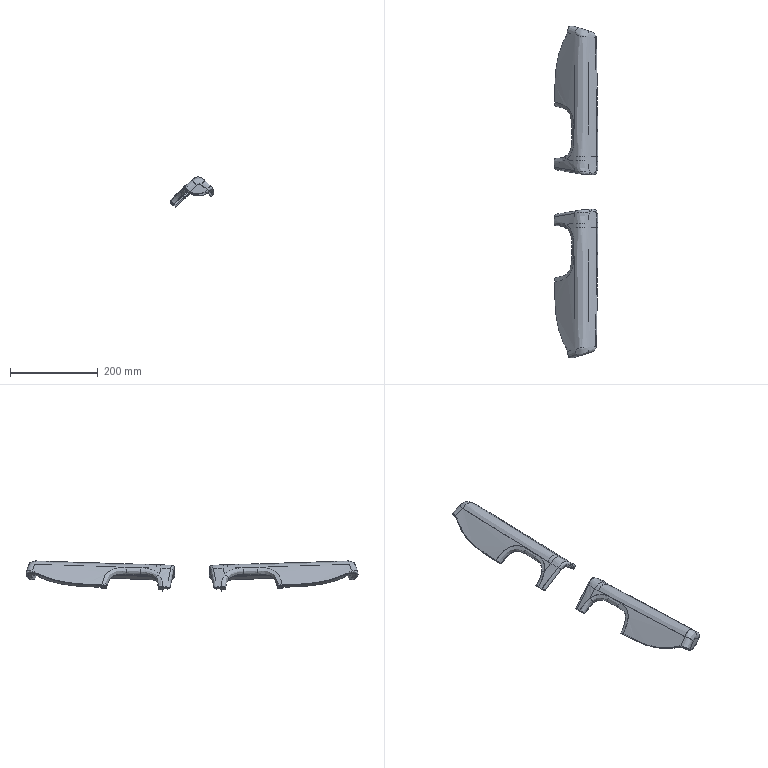Part | STEP file | L0193019AA ARMREST FRT DR MANUAL RH!SKIN VINYL ARMREST FRONT DOOR RH MANUAL | 2 solids | 636 faces | box 99.664 x 758.37 x 68.586 mm | volume 134789 mm3 | spline 618 | plane 18